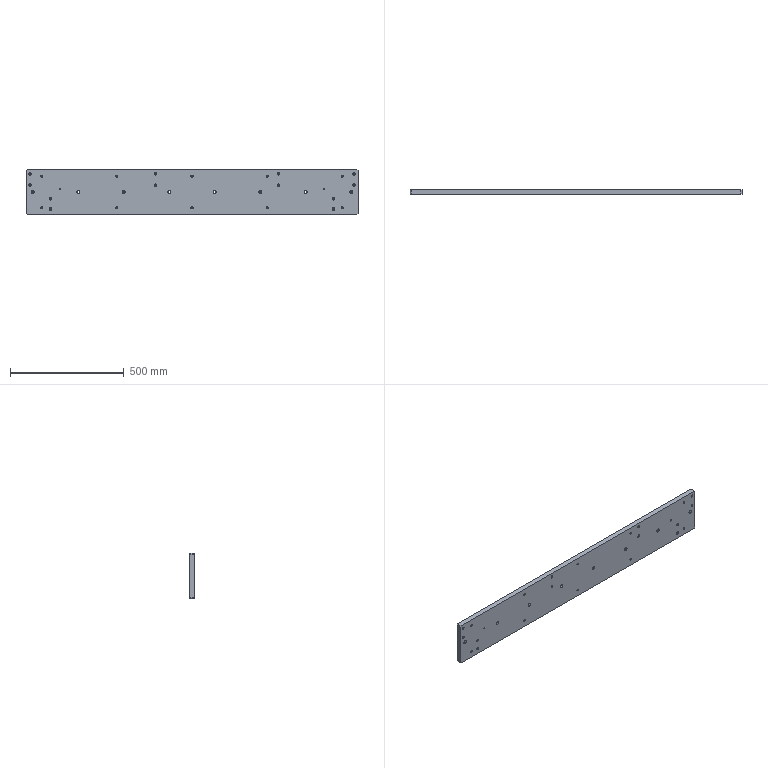Part | STEP file | ND25021-01-JDKM-01-TL | 1 solid | 170 faces | box 1460 x 20 x 200 mm | volume 5782865 mm3 | cylinder 128 | plane 42 | commonest cylinder face diameters 15 x36 6.6 x24 11 x24 9 x20 10 x16 6 x4